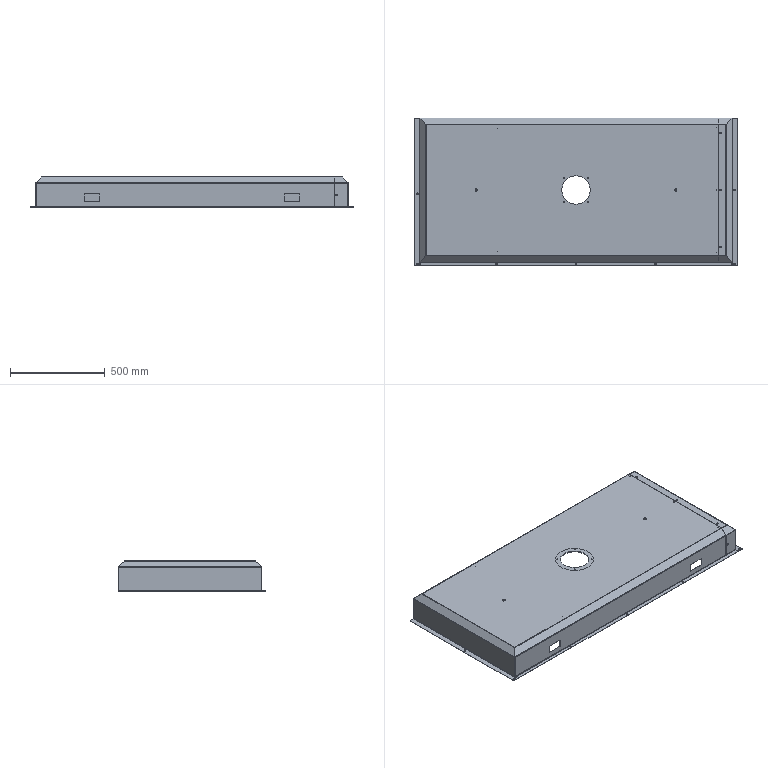Part | NX | features solid 2 | 1 solid | 219 faces | box 1702 x 776.8 x 160 mm | volume 2466144 mm3 | cylinder 104 | plane 99 | spline 16 | commonest cylinder face diameters 10 x34 2.4 x16 4.8 x16 8 x12 1 x10 5.188 x8